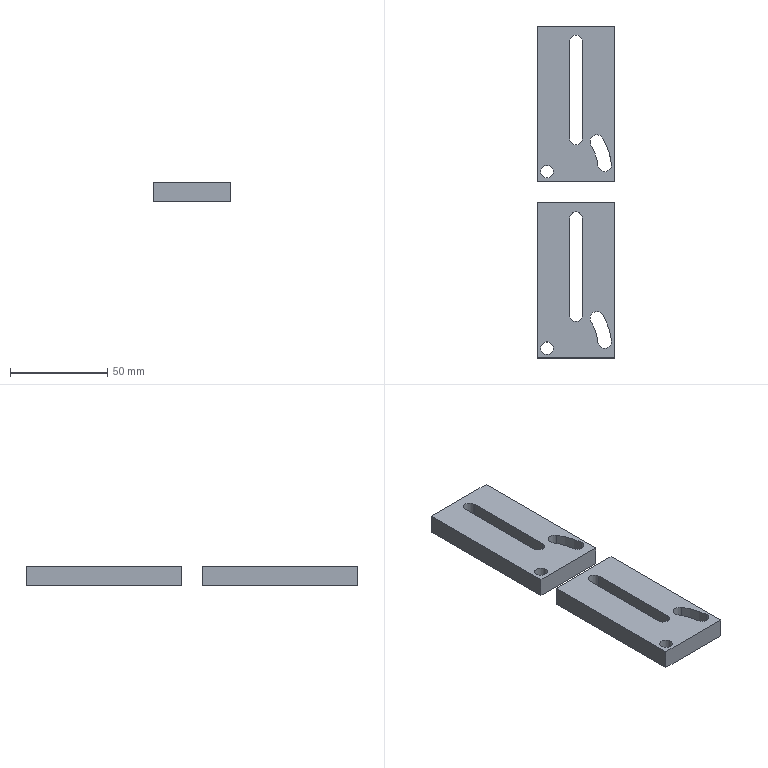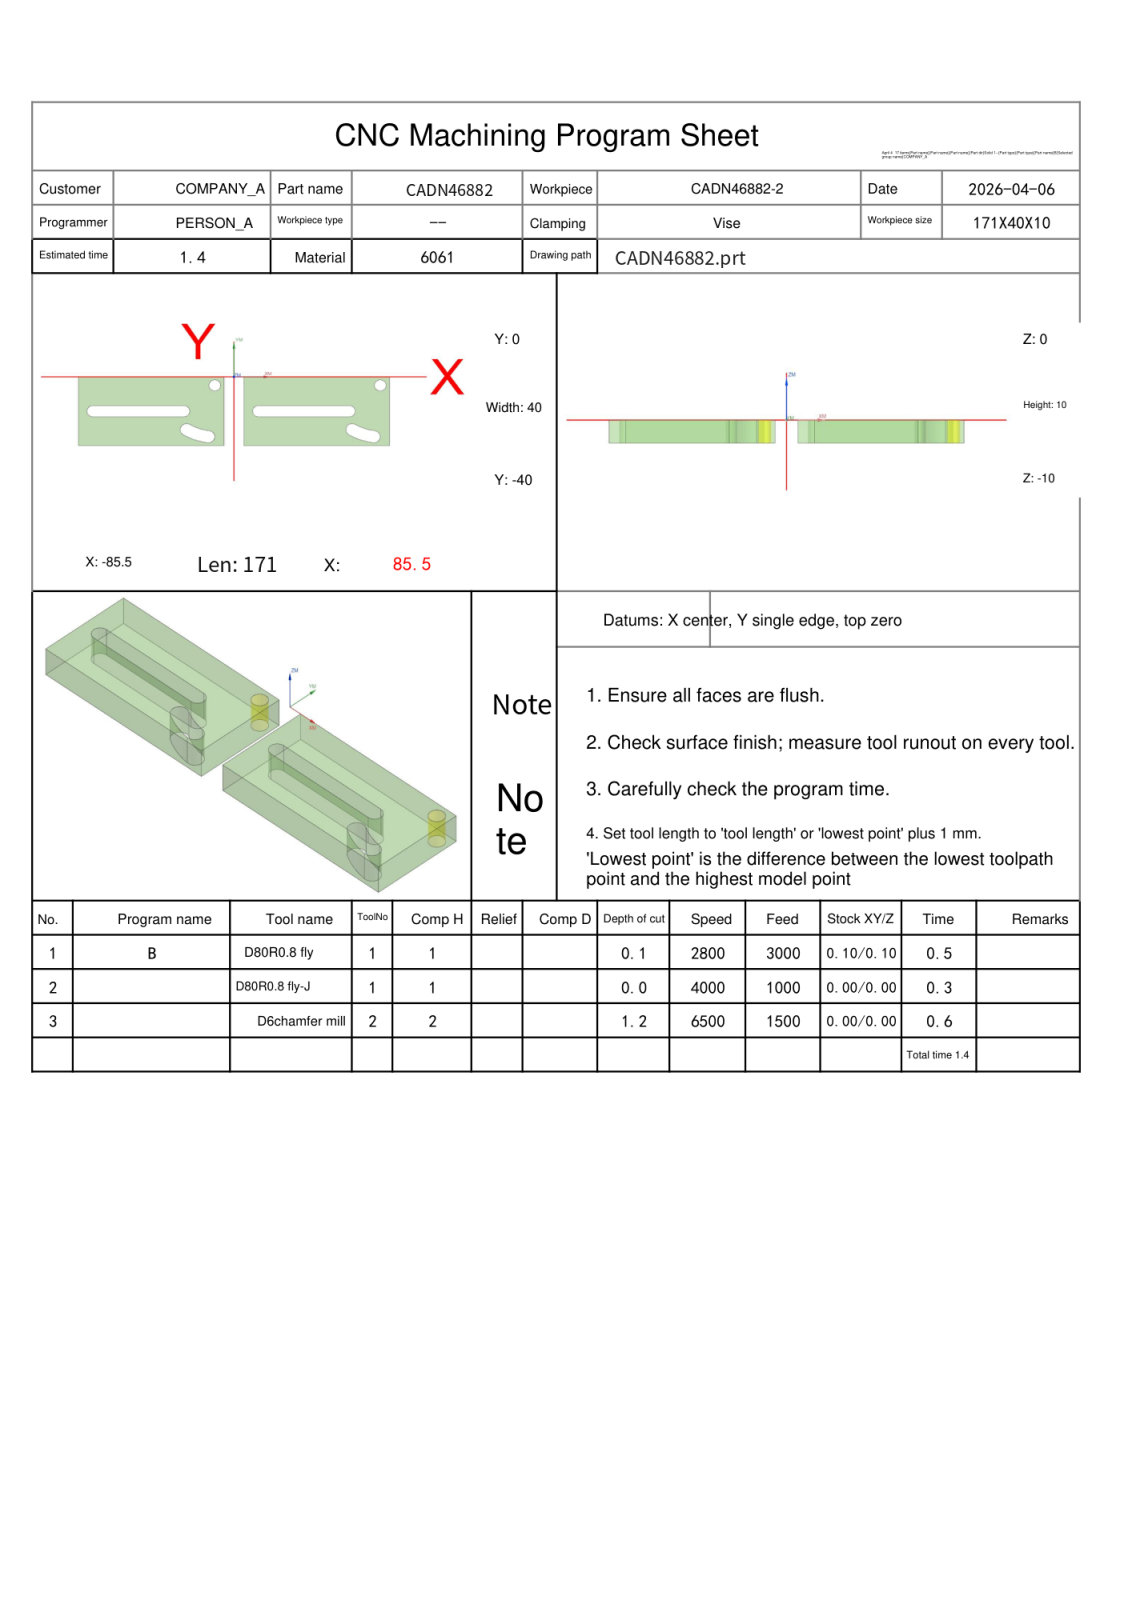NC program | NX | posted by the shop | part box 40 x 171 x 10 mm
Whole program:
%
O0001
(Machine time: 1.95 MIN)
(===Total Tool:2===)
(T1=D80R0.8 fly D=80.  R=0.8  D-  H01 Z=0.    )
(T2=D6chamfer mill   D=6.   R=0.   D-  H02 Z=-1.2  )
G80 G90 G17 G49 G40
G91 G28 Z0
M01
N1 T01 M06
(D80R0.8 fly  D=80. R=0.8 H=01 ce=0.10 di=0.10)
G00 G90 G54 X137.597 Y-20. M03 S2800
G43 H01 Z20.
M08
Z3.525
G01 Z1.525 F3000.
X125.597
X-125.597
X-137.597
Z3.525
G00 X137.597
Z3.05
G01 Z1.05
X125.597
X-125.597
X-137.597
Z3.05
G00 X137.597
Z2.575
G01 Z.575
X125.597
X-125.597
X-137.597
Z2.575
G00 X137.597
Z2.1
G01 Z.1
X125.597
X-125.597
X-137.597
Z2.1
G00 Z20.
G91 G28 Z0.0
M05
M09
G91 G28 Z0.0
M01
N2 T01 M06
(D80R0.8 fly-J  D=80. R=0.8 H=01 ce=0.00 di=0.00)
G00 G90 G54 X137.499 Y-20. M03 S4000
G43 H01 Z20.
M08
Z2.
G01 Z0.0 F1000.
X125.499
X-125.499
X-137.499
Z2.
G00 Z20.
G91 G28 Z0.0
M05
M09
G91 G28 Z0.0
M01
N3 T02 M06
(D6chamfer mill  D=6. R=0. H=02 ce=0.00 di=0.00)
G00 G90 G54 X-45.114 Y-41.227 M03 S6500
G43 H02 Z20.
M08
Z.172
G01 Z-1.2 F1500.
G03 X-45.4 Y-41.027 I-1.286 J-1.532
G01 X-45.446 Y-40.997
X-45.5 Y-41.
X-85.5
G02 X-86.5 Y-40. I0.0 J1.
G01 Y0.0
G02 X-85.5 Y1. I1. J0.0
G01 X-5.5
G02 X-4.5 Y0.0 I0.0 J-1.
G01 Y-40.
G02 X-5.5 Y-41. I-1. J0.0
G01 X-45.5
X-45.554 Y-40.997
X-45.6 Y-41.027
G03 X-45.886 Y-41.227 I1. J-1.732
G01 Z.172
G00 Z10.
X-52.114 Y-17.977
Z.172
G01 Z-1.2
G03 X-52.4 Y-17.777 I-1.286 J-1.532
G01 X-52.446 Y-17.747
X-52.5 Y-17.75
X-77.5
G03 X-79.75 Y-20. I0.0 J-2.25
X-77.5 Y-22.25 I2.25 J0.0
G01 X-27.5
G03 X-25.25 Y-20. I0.0 J2.25
X-27.5 Y-17.75 I-2.25 J0.0
G01 X-52.5
X-52.554 Y-17.747
X-52.6 Y-17.777
G03 X-52.886 Y-17.977 I1. J-1.732
G01 Z.172
G00 Z10.
X-21.304 Y-35.423
Z.189
G01 Z-1.2
G03 X-21.092 Y-35.7 I1.689 J1.07
G01 X-21.058 Y-35.742
X-21.005 Y-35.755
G03 X-14.292 Y-37.278 I10.505 J30.755
X-14. Y-37.295 I.292 J2.483
X-11.5 Y-34.795 I0.0 J2.5
X-13.708 Y-32.312 I-2.5 J0.0
G02 X-24.67 Y-28.568 I3.208 J27.312
G03 X-25.959 Y-28.211 I-1.288 J-2.143
X-28.459 Y-30.711 I0.0 J-2.5
X-27.247 Y-32.853 I2.5 J0.0
X-21.005 Y-35.755 I16.747 J27.853
G01 X-20.955 Y-35.777
X-20.902 Y-35.765
G03 X-20.565 Y-35.675 I-.345 J1.97
G01 Z.189
G00 Z10.
X-10.096 Y-2.942
Z.253
G01 Z-1.2
G03 X-10.398 Y-2.768 I-1.147 J-1.638
G01 X-10.446 Y-2.742
X-10.5 Y-2.75
G03 X-12.75 Y-5. I0.0 J-2.25
X-10.5 Y-7.25 I2.25 J0.0
X-8.25 Y-5. I0.0 J2.25
X-10.5 Y-2.75 I-2.25 J0.0
G01 X-10.554 Y-2.742
X-10.602 Y-2.768
G03 X-10.904 Y-2.942 I.845 J-1.813
G01 Z.253
G00 Z10.
X45.886 Y-41.227
Z.172
G01 Z-1.2
G03 X45.6 Y-41.027 I-1.286 J-1.532
G01 X45.554 Y-40.997
X45.5 Y-41.
X5.5
G02 X4.5 Y-40. I0.0 J1.
G01 Y0.0
G02 X5.5 Y1. I1. J0.0
G01 X85.5
G02 X86.5 Y0.0 I0.0 J-1.
G01 Y-40.
G02 X85.5 Y-41. I-1. J0.0
G01 X45.5
X45.446 Y-40.997
X45.4 Y-41.027
G03 X45.114 Y-41.227 I1. J-1.732
G01 Z.172
G00 Z10.
X38.886 Y-17.977
Z.172
G01 Z-1.2
G03 X38.6 Y-17.777 I-1.286 J-1.532
G01 X38.554 Y-17.747
X38.5 Y-17.75
X13.5
G03 X11.25 Y-20. I0.0 J-2.25
X13.5 Y-22.25 I2.25 J0.0
G01 X63.5
G03 X65.75 Y-20. I0.0 J2.25
X63.5 Y-17.75 I-2.25 J0.0
G01 X38.5
X38.446 Y-17.747
X38.4 Y-17.777
G03 X38.114 Y-17.977 I1. J-1.732
G01 Z.172
G00 Z10.
X69.696 Y-35.423
Z.189
G01 Z-1.2
G03 X69.908 Y-35.7 I1.689 J1.07
G01 X69.942 Y-35.742
X69.995 Y-35.755
G03 X76.708 Y-37.278 I10.505 J30.755
X77. Y-37.295 I.292 J2.483
X79.5 Y-34.795 I0.0 J2.5
X77.292 Y-32.312 I-2.5 J0.0
G02 X66.33 Y-28.568 I3.208 J27.312
G03 X65.041 Y-28.211 I-1.288 J-2.143
X62.541 Y-30.711 I0.0 J-2.5
X63.753 Y-32.853 I2.5 J0.0
X69.995 Y-35.755 I16.747 J27.853
G01 X70.045 Y-35.777
X70.098 Y-35.765
G03 X70.435 Y-35.675 I-.345 J1.97
G01 Z.189
G00 Z10.
X80.904 Y-2.942
Z.253
G01 Z-1.2
G03 X80.602 Y-2.768 I-1.147 J-1.638
G01 X80.554 Y-2.742
X80.5 Y-2.75
G03 X78.25 Y-5. I0.0 J-2.25
X80.5 Y-7.25 I2.25 J0.0
X82.75 Y-5. I0.0 J2.25
X80.5 Y-2.75 I-2.25 J0.0
G01 X80.446 Y-2.742
X80.398 Y-2.768
G03 X80.096 Y-2.942 I.845 J-1.813
G01 Z.253
G00 Z20.
M05
M09
G91 G28 Z0.0
G91 G28 Y0.0
M30
%